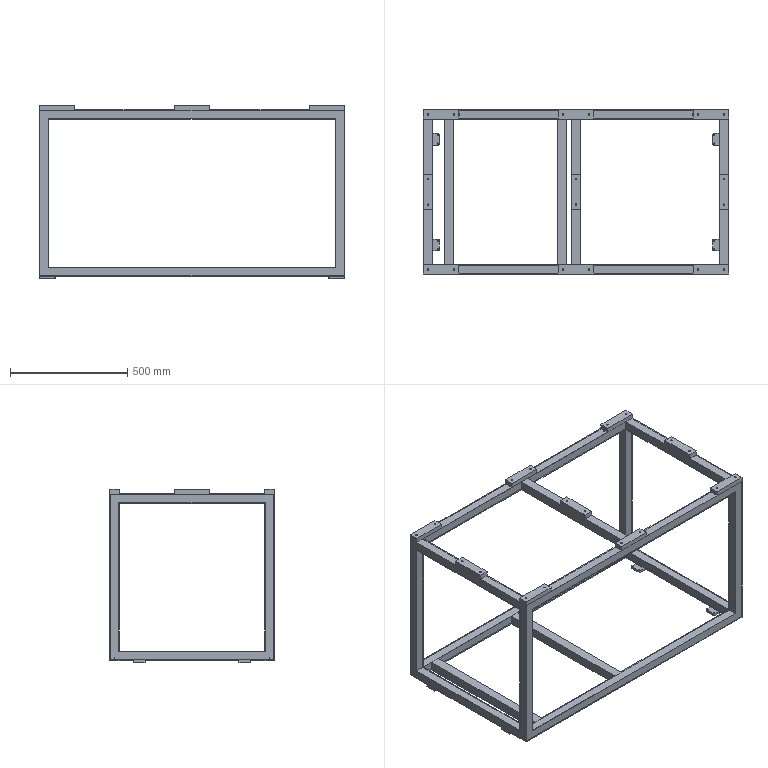Part | SolidWorks | features ICE 11, MirrorPattern 9, HoleWzd 5, LPattern 5, 3DProfileFeature 4, Chamfer 1, Extrusion 1, Shell 1 | 1 solid | 319 faces | box 1300 x 700 x 740 mm | volume 7989139 mm3 | plane 169 | cylinder 98 | cone 52 | commonest cylinder face diameters 6.8 x36 5 x32 4.2 x16 16 x8 8 x6